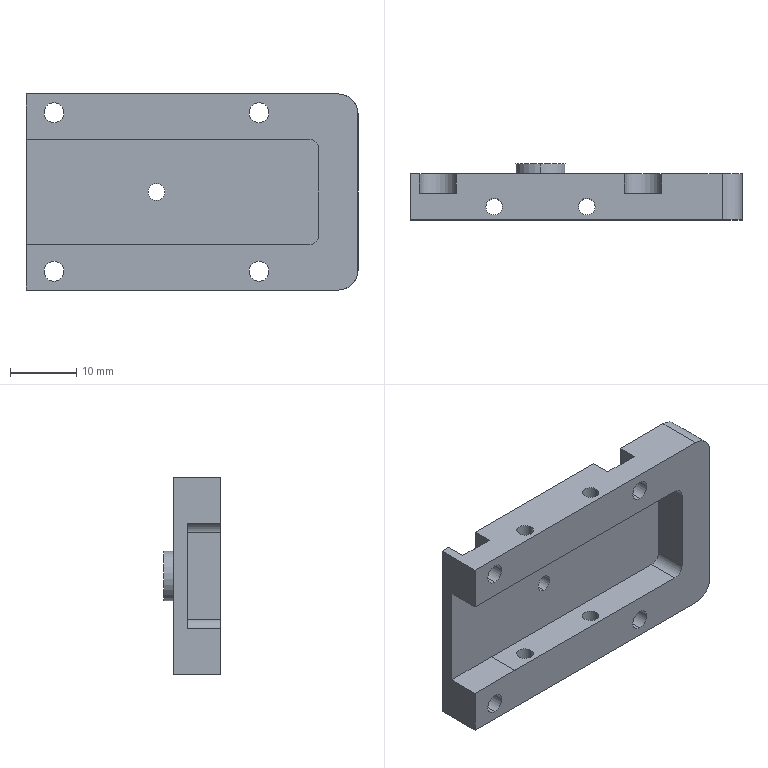Part | NX | features BREP 1 | 1 solid | 58 faces | box 50.135 x 8.5 x 29.6 mm | volume 6295 mm3 | cylinder 34 | plane 24 | commonest cylinder face diameters 3 x13 2.5 x10 5.6 x6 6 x3 7.5 x2